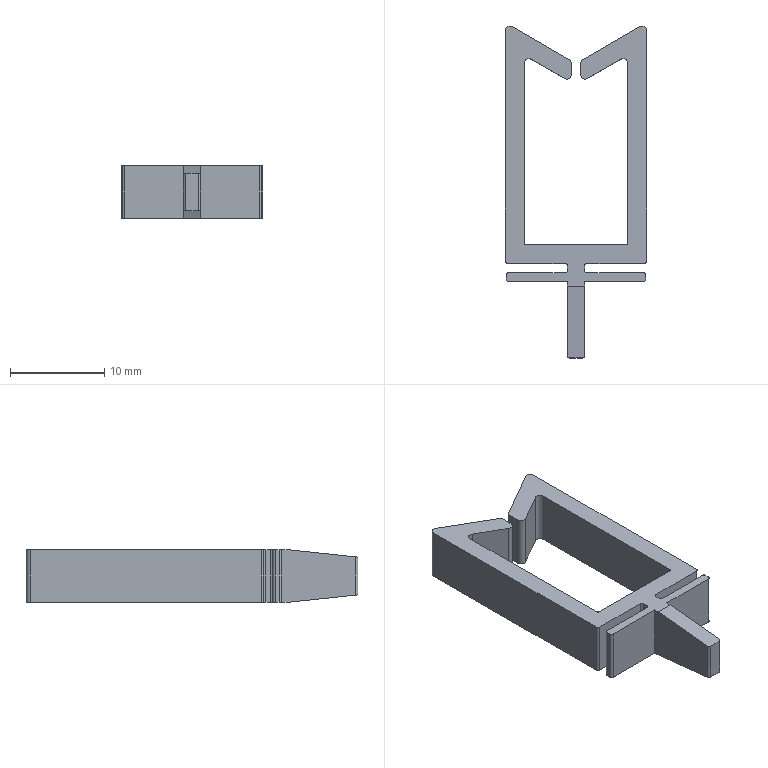Part | STEP file | 10007151 | 1 solid | 50 faces | box 15 x 35.134 x 5.6 mm | volume 963.979 mm3 | plane 28 | cylinder 22 | commonest cylinder face diameters 0.5 x14 1 x8